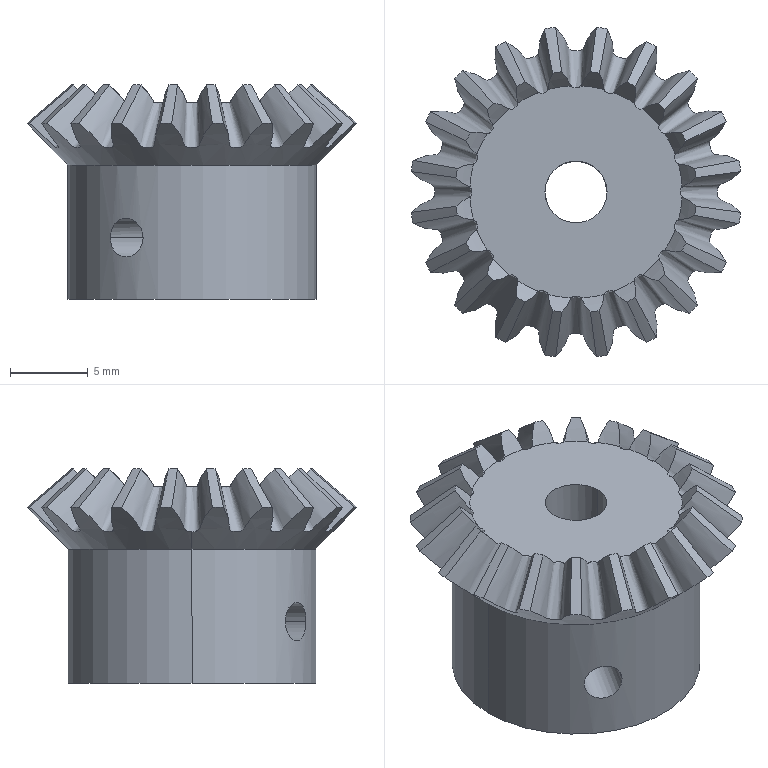Part | SolidWorks | features 3DProfileFeature 9, ICE 2, BlendCut 1, CirPattern 1, CurveInFile 1, HoleWzd 1, RefAxis 1, RevCut 1, Revolution 1 | 1 solid | 74 faces | box 21.253 x 21.253 x 13.804 mm | volume 2568 mm3 | cone 44 | spline 20 | cylinder 8 | plane 2 | commonest cylinder face diameters 2.5 x4 4 x2 16 x2